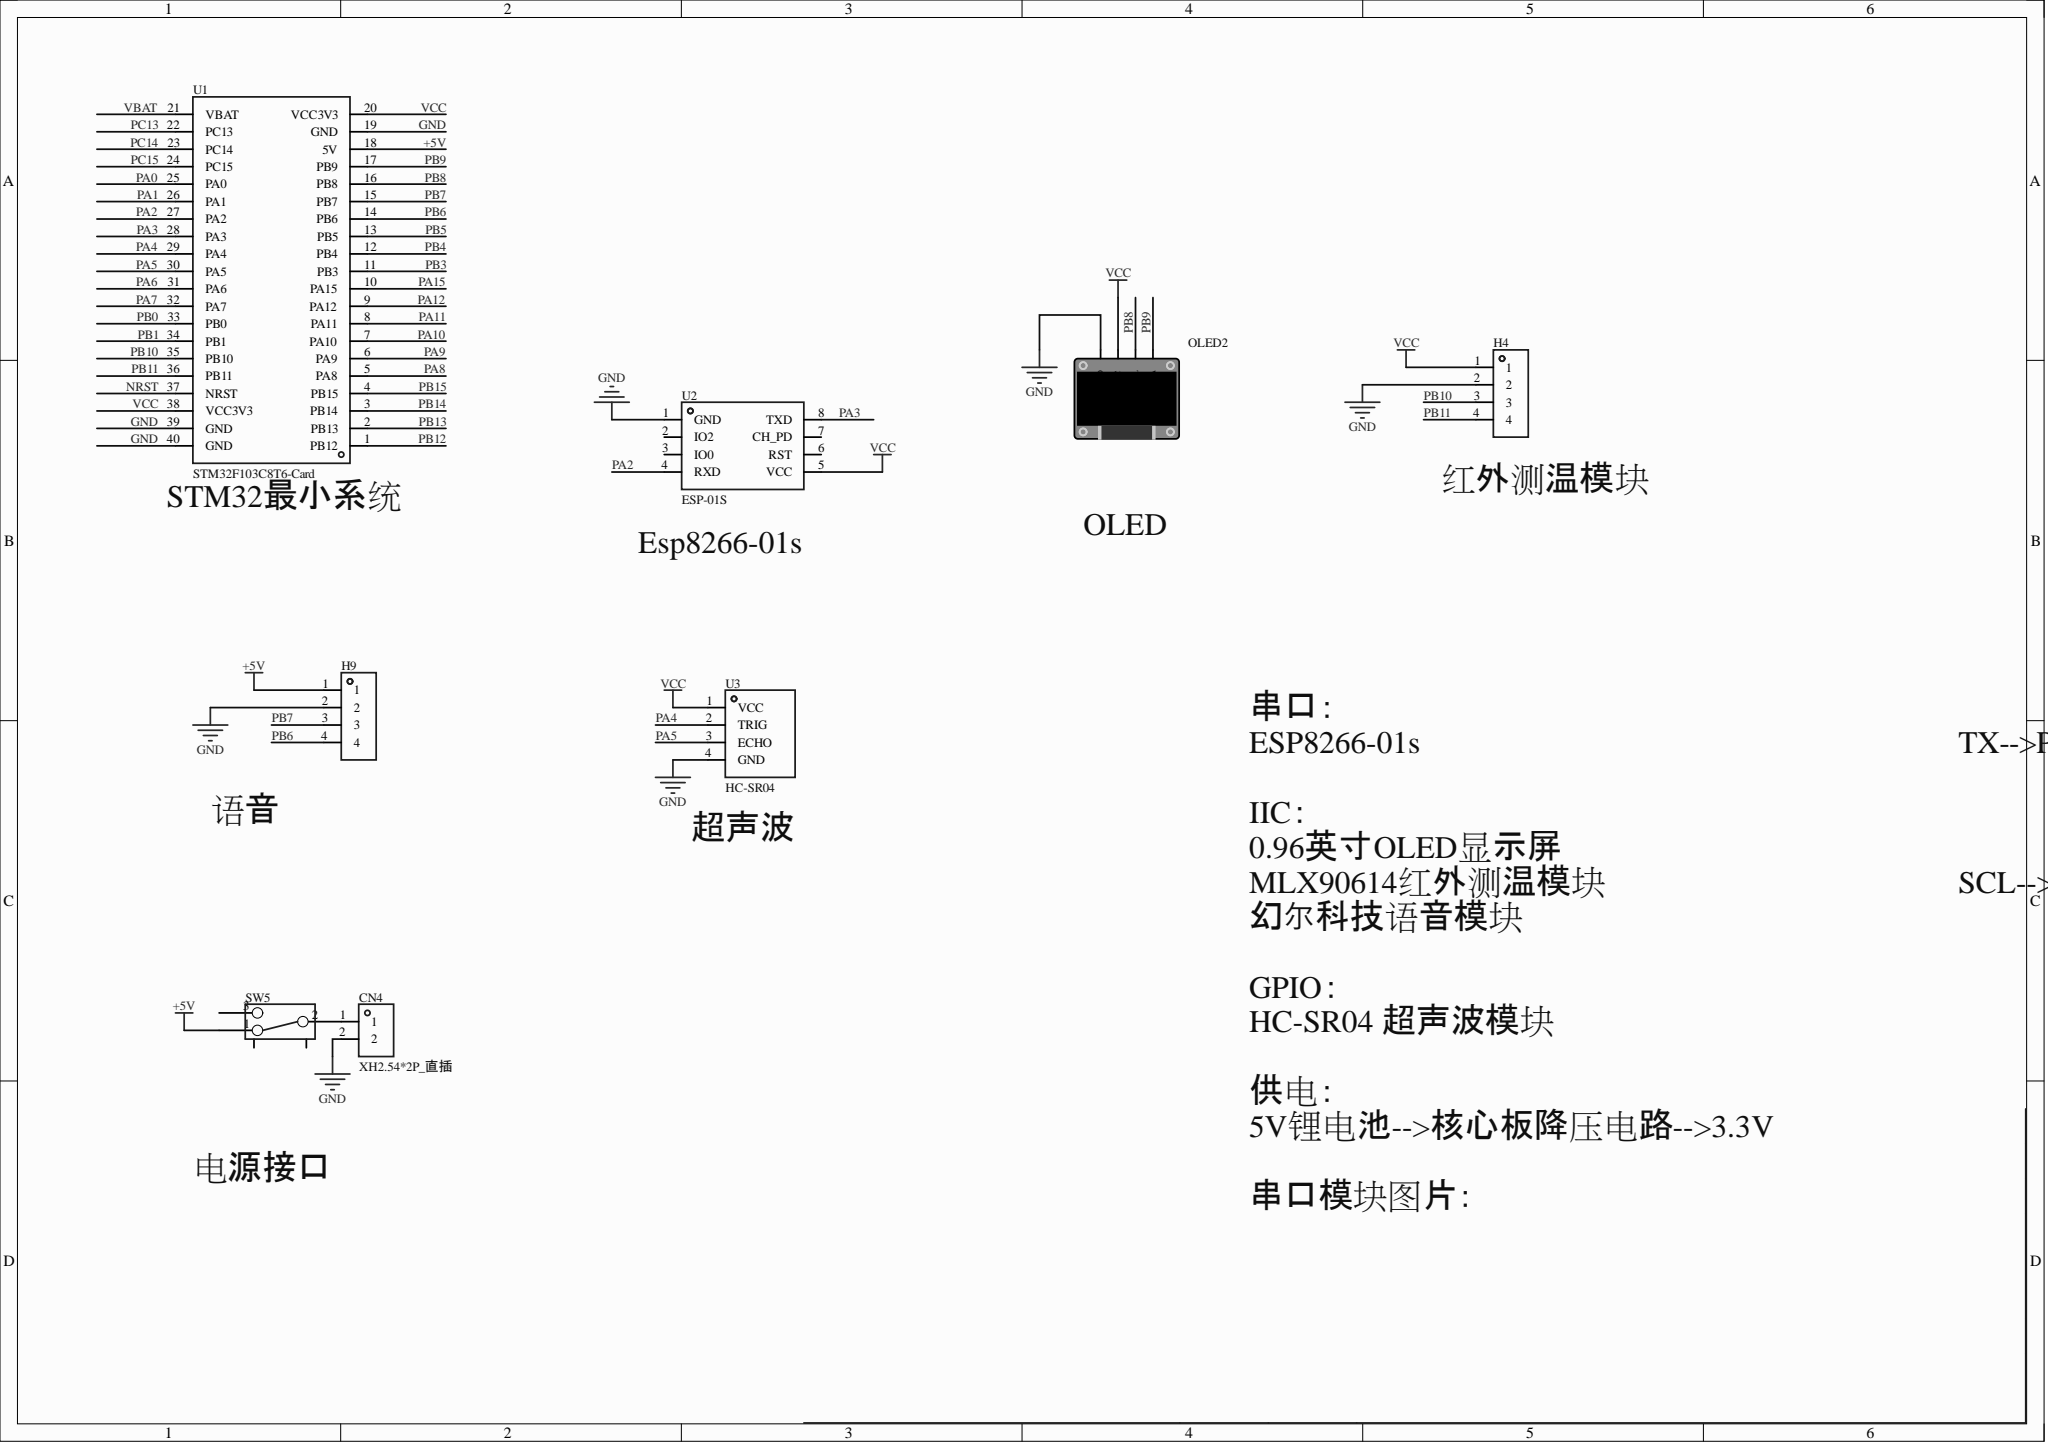Circuit board | Altium Designer | 8 parts | 14 nets
Bill of materials:
Comment,Description,Designator,Footprint,LibRef,Quantity
"XH2.54*2P_直插","","CN4","CONN-TH_2P-P2.50-XH2.54-2P","XH2.54*2P_直插","1"
"","","H4, H9","HDR-TH_4P-P2.54-V-F","HDR-F_2.54_1x4P","2"
"","","OLED2","0.96OLED_4P","0.96OLED模块_4P","1"
"","","SW5","拨动开关","拨动开关_正","1"
"STM32F103C8T6-Card","","U1","CONN-TH_L53.3-W22.9_STM32F103C8T6-CARD","STM32F103C8T6-Card","1"
"ESP-01S","","U2","WIFIM-TH_ESP-01S","ESP-01S_C111009","1"
"HC-SR04","","U3","TH_HC-SR04V","HC-SR04","1"
Netlist (Protel format):
[
CN4
CONN-TH_2P-P2.50-XH2.54-2P
XH2.54*2P_直插



]
[
H4
HDR-TH_4P-P2.54-V-F




]
[
H9
HDR-TH_4P-P2.54-V-F




]
[
OLED2
0.96OLED_4P




]
[
SW5
拨动开关




]
[
U1
CONN-TH_L53.3-W22.9_STM32F103C8T6-CARD
STM32F103C8T6-Card



]
[
U2
WIFIM-TH_ESP-01S
ESP-01S



]
[
U3
TH_HC-SR04V
HC-SR04



]
(
VCC
H4-1
OLED2-2
U1-20
U1-38
U2-5
U3-1
)
(
PB11
H4-4
U1-36
)
(
PB10
H4-3
U1-35
)
(
PB9
OLED2-4
U1-17
)
(
PB8
OLED2-3
U1-16
)
(
PB7
H9-3
U1-15
)
(
PB6
H9-4
U1-14
)
(
PA5
U1-30
U3-3
)
(
PA4
U1-29
U3-2
)
(
PA3
U1-28
U2-8
)
(
PA2
U1-27
U2-4
)
(
NetCN4_1
CN4-1
SW5-2
)
(
GND
CN4-2
H4-2
H9-2
OLED2-1
U1-19
U1-39
U1-40
U2-1
U3-4
)
(
+5V
H9-1
SW5-1
U1-18
)